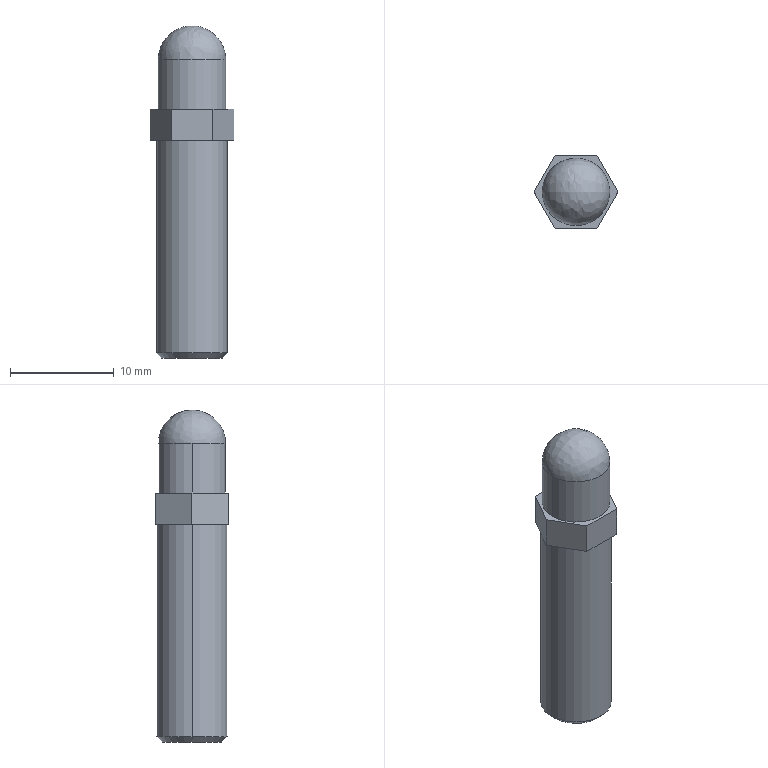Part | STEP file | Product upper | 1 solid | 16 faces | box 8.083 x 7 x 31.87 mm | volume 1117 mm3 | plane 9 | cylinder 4 | cone 2 | spline 1 | commonest cylinder face diameters 6.5 x2 6.8 x2
STEP:
#1=CARTESIAN_POINT('',(0.,0.,0.));
#2=DIRECTION('',(0.,0.,1.));
#3=DIRECTION('',(1.,0.,0.));
#4=AXIS2_PLACEMENT_3D('',#1,#2,#3);
#5=CARTESIAN_POINT('',(3.4,0.,-20.5));
#6=VERTEX_POINT('',#5);
#7=CARTESIAN_POINT('',(-3.4,0.,-20.5));
#8=VERTEX_POINT('',#7);
#9=CARTESIAN_POINT('',(0.,0.,-20.5));
#10=DIRECTION('',(0.,0.,1.));
#11=DIRECTION('',(1.,0.,0.));
#12=AXIS2_PLACEMENT_3D('',#9,#10,#11);
#13=CIRCLE('',#12,3.4);
#14=CARTESIAN_POINT('',(0.,0.,-21.));
#15=DIRECTION('',(0.,0.,1.));
#16=DIRECTION('',(1.,0.,0.));
#17=AXIS2_PLACEMENT_3D('',#14,#15,#16);
#18=CYLINDRICAL_SURFACE('',#17,3.4);
#19=CARTESIAN_POINT('',(0.,0.5));
#20=DIRECTION('',(1.,0.));
#21=VECTOR('',#20,1.);
#22=LINE('',#19,#21);
#23=(GEOMETRIC_REPRESENTATION_CONTEXT(2)PARAMETRIC_REPRESENTATION_CONTEXT()REPRESENTATION_CONTEXT('',''));
#24=DEFINITIONAL_REPRESENTATION('',(#22),#23);
#25=PCURVE('',#18,#24);
#26=CARTESIAN_POINT('',(0.,0.,-20.5));
#27=DIRECTION('',(0.,0.,1.));
#28=DIRECTION('',(1.,0.,0.));
#29=AXIS2_PLACEMENT_3D('',#26,#27,#28);
#30=CONICAL_SURFACE('',#29,3.4,0.7854);
#31=CARTESIAN_POINT('',(0.,0.));
#32=DIRECTION('',(1.,0.));
#33=VECTOR('',#32,1.);
#34=LINE('',#31,#33);
#35=(GEOMETRIC_REPRESENTATION_CONTEXT(2)PARAMETRIC_REPRESENTATION_CONTEXT()REPRESENTATION_CONTEXT('',''));
#36=DEFINITIONAL_REPRESENTATION('',(#34),#35);
#37=PCURVE('',#30,#36);
#38=SURFACE_CURVE('',#13,(#25,#37),.PCURVE_S1.);
#39=EDGE_CURVE('',#6,#8,#38,.T.);
#40=ORIENTED_EDGE('',*,*,#39,.T.);
#41=CARTESIAN_POINT('',(-3.4,0.,0.));
#42=VERTEX_POINT('',#41);
#43=CARTESIAN_POINT('',(-3.4,0.,-21.));
#44=DIRECTION('',(0.,0.,1.));
#45=VECTOR('',#44,1.);
#46=LINE('',#43,#45);
#47=CARTESIAN_POINT('',(3.142,0.));
#48=DIRECTION('',(0.,1.));
#49=VECTOR('',#48,1.);
#50=LINE('',#47,#49);
#51=(GEOMETRIC_REPRESENTATION_CONTEXT(2)PARAMETRIC_REPRESENTATION_CONTEXT()REPRESENTATION_CONTEXT('',''));
#52=DEFINITIONAL_REPRESENTATION('',(#50),#51);
#53=PCURVE('',#18,#52);
#54=CARTESIAN_POINT('',(0.,0.,-21.));
#55=DIRECTION('',(0.,0.,1.));
#56=DIRECTION('',(1.,0.,0.));
#57=AXIS2_PLACEMENT_3D('',#54,#55,#56);
#58=CYLINDRICAL_SURFACE('',#57,3.4);
#59=CARTESIAN_POINT('',(3.142,0.));
#60=DIRECTION('',(0.,1.));
#61=VECTOR('',#60,1.);
#62=LINE('',#59,#61);
#63=(GEOMETRIC_REPRESENTATION_CONTEXT(2)PARAMETRIC_REPRESENTATION_CONTEXT()REPRESENTATION_CONTEXT('',''));
#64=DEFINITIONAL_REPRESENTATION('',(#62),#63);
#65=PCURVE('',#58,#64);
#66=SURFACE_CURVE('',#46,(#53,#65),.PCURVE_S1.);
#67=EDGE_CURVE('',#8,#42,#66,.T.);
#68=ORIENTED_EDGE('',*,*,#67,.T.);
#69=CARTESIAN_POINT('',(3.4,0.,0.));
#70=VERTEX_POINT('',#69);
#71=CARTESIAN_POINT('',(0.,0.,0.));
#72=DIRECTION('',(0.,0.,-1.));
#73=DIRECTION('',(1.,0.,0.));
#74=AXIS2_PLACEMENT_3D('',#71,#72,#73);
#75=CIRCLE('',#74,3.4);
#76=CARTESIAN_POINT('',(6.283,21.));
#77=DIRECTION('',(-1.,0.));
#78=VECTOR('',#77,1.);
#79=LINE('',#76,#78);
#80=(GEOMETRIC_REPRESENTATION_CONTEXT(2)PARAMETRIC_REPRESENTATION_CONTEXT()REPRESENTATION_CONTEXT('',''));
#81=DEFINITIONAL_REPRESENTATION('',(#79),#80);
#82=PCURVE('',#18,#81);
#83=CARTESIAN_POINT('',(0.,0.,0.));
#84=DIRECTION('',(0.,0.,1.));
#85=DIRECTION('',(1.,0.,0.));
#86=AXIS2_PLACEMENT_3D('',#83,#84,#85);
#87=PLANE('',#86);
#88=CARTESIAN_POINT('',(3.4,0.));
#89=CARTESIAN_POINT('',(3.4,-5.889));
#90=CARTESIAN_POINT('',(-1.7,-2.944));
#91=CARTESIAN_POINT('',(-6.8,0.));
#92=CARTESIAN_POINT('',(-1.7,2.944));
#93=CARTESIAN_POINT('',(3.4,5.889));
#94=CARTESIAN_POINT('',(3.4,0.));
#95=(BOUNDED_CURVE()B_SPLINE_CURVE(2,(#88,#89,#90,#91,#92,#93,#94),.UNSPECIFIED.,.T.,.F.)B_SPLINE_CURVE_WITH_KNOTS((1,2,2,2,2,1),(-2.094,0.,2.094,4.189,6.283,8.378),.UNSPECIFIED.)CURVE()GEOMETRIC_REPRESENTATION_ITEM()RATIONAL_B_SPLINE_CURVE((1.,0.5,1.,0.5,1.,0.5,1.))REPRESENTATION_ITEM(''));
#96=(GEOMETRIC_REPRESENTATION_CONTEXT(2)PARAMETRIC_REPRESENTATION_CONTEXT()REPRESENTATION_CONTEXT('',''));
#97=DEFINITIONAL_REPRESENTATION('',(#95),#96);
#98=PCURVE('',#87,#97);
#99=SURFACE_CURVE('',#75,(#82,#98),.PCURVE_S1.);
#100=EDGE_CURVE('',#42,#70,#99,.T.);
#101=ORIENTED_EDGE('',*,*,#100,.T.);
#102=CARTESIAN_POINT('',(3.4,0.,-21.));
#103=DIRECTION('',(0.,0.,1.));
#104=VECTOR('',#103,1.);
#105=LINE('',#102,#104);
#106=CARTESIAN_POINT('',(0.,0.));
#107=DIRECTION('',(0.,1.));
#108=VECTOR('',#107,1.);
#109=LINE('',#106,#108);
#110=(GEOMETRIC_REPRESENTATION_CONTEXT(2)PARAMETRIC_REPRESENTATION_CONTEXT()REPRESENTATION_CONTEXT('',''));
#111=DEFINITIONAL_REPRESENTATION('',(#109),#110);
#112=PCURVE('',#18,#111);
#113=CARTESIAN_POINT('',(6.283,0.));
#114=DIRECTION('',(0.,1.));
#115=VECTOR('',#114,1.);
#116=LINE('',#113,#115);
#117=(GEOMETRIC_REPRESENTATION_CONTEXT(2)PARAMETRIC_REPRESENTATION_CONTEXT()REPRESENTATION_CONTEXT('',''));
#118=DEFINITIONAL_REPRESENTATION('',(#116),#117);
#119=PCURVE('',#58,#118);
#120=SURFACE_CURVE('',#105,(#112,#119),.PCURVE_S1.);
#121=EDGE_CURVE('',#6,#70,#120,.T.);
#122=ORIENTED_EDGE('',*,*,#121,.F.);
#123=EDGE_LOOP('',(#40,#68,#101,#122));
#124=FACE_BOUND('',#123,.T.);
#125=ADVANCED_FACE('',(#124),#18,.T.);
#126=CARTESIAN_POINT('',(2.9,0.,-21.));
#127=VERTEX_POINT('',#126);
#128=CARTESIAN_POINT('',(-2.9,0.,-21.));
#129=VERTEX_POINT('',#128);
#130=CARTESIAN_POINT('',(0.,0.,-21.));
#131=DIRECTION('',(0.,0.,1.));
#132=DIRECTION('',(1.,0.,0.));
#133=AXIS2_PLACEMENT_3D('',#130,#131,#132);
#134=CIRCLE('',#133,2.9);
#135=CARTESIAN_POINT('',(0.,-0.5));
#136=DIRECTION('',(1.,0.));
#137=VECTOR('',#136,1.);
#138=LINE('',#135,#137);
#139=(GEOMETRIC_REPRESENTATION_CONTEXT(2)PARAMETRIC_REPRESENTATION_CONTEXT()REPRESENTATION_CONTEXT('',''));
#140=DEFINITIONAL_REPRESENTATION('',(#138),#139);
#141=PCURVE('',#30,#140);
#142=CARTESIAN_POINT('',(0.,0.,-21.));
#143=DIRECTION('',(0.,0.,-1.));
#144=DIRECTION('',(-1.,0.,0.));
#145=AXIS2_PLACEMENT_3D('',#142,#143,#144);
#146=PLANE('',#145);
#147=CARTESIAN_POINT('',(-2.9,0.));
#148=CARTESIAN_POINT('',(-2.9,5.023));
#149=CARTESIAN_POINT('',(1.45,2.511));
#150=CARTESIAN_POINT('',(5.8,0.));
#151=CARTESIAN_POINT('',(1.45,-2.511));
#152=CARTESIAN_POINT('',(-2.9,-5.023));
#153=CARTESIAN_POINT('',(-2.9,0.));
#154=(BOUNDED_CURVE()B_SPLINE_CURVE(2,(#147,#148,#149,#150,#151,#152,#153),.UNSPECIFIED.,.T.,.F.)B_SPLINE_CURVE_WITH_KNOTS((1,2,2,2,2,1),(-2.094,0.,2.094,4.189,6.283,8.378),.UNSPECIFIED.)CURVE()GEOMETRIC_REPRESENTATION_ITEM()RATIONAL_B_SPLINE_CURVE((1.,0.5,1.,0.5,1.,0.5,1.))REPRESENTATION_ITEM(''));
#155=(GEOMETRIC_REPRESENTATION_CONTEXT(2)PARAMETRIC_REPRESENTATION_CONTEXT()REPRESENTATION_CONTEXT('',''));
#156=DEFINITIONAL_REPRESENTATION('',(#154),#155);
#157=PCURVE('',#146,#156);
#158=SURFACE_CURVE('',#134,(#141,#157),.PCURVE_S1.);
#159=EDGE_CURVE('',#127,#129,#158,.T.);
#160=ORIENTED_EDGE('',*,*,#159,.T.);
#161=CARTESIAN_POINT('',(-3.4,0.,-20.5));
#162=DIRECTION('',(-0.7071,0.,0.7071));
#163=VECTOR('',#162,1.);
#164=LINE('',#161,#163);
#165=CARTESIAN_POINT('',(3.142,0.));
#166=DIRECTION('',(0.,1.));
#167=VECTOR('',#166,1.);
#168=LINE('',#165,#167);
#169=(GEOMETRIC_REPRESENTATION_CONTEXT(2)PARAMETRIC_REPRESENTATION_CONTEXT()REPRESENTATION_CONTEXT('',''));
#170=DEFINITIONAL_REPRESENTATION('',(#168),#169);
#171=PCURVE('',#30,#170);
#172=CARTESIAN_POINT('',(0.,0.,-20.5));
#173=DIRECTION('',(0.,0.,1.));
#174=DIRECTION('',(1.,0.,0.));
#175=AXIS2_PLACEMENT_3D('',#172,#173,#174);
#176=CONICAL_SURFACE('',#175,3.4,0.7854);
#177=CARTESIAN_POINT('',(3.142,0.));
#178=DIRECTION('',(0.,1.));
#179=VECTOR('',#178,1.);
#180=LINE('',#177,#179);
#181=(GEOMETRIC_REPRESENTATION_CONTEXT(2)PARAMETRIC_REPRESENTATION_CONTEXT()REPRESENTATION_CONTEXT('',''));
#182=DEFINITIONAL_REPRESENTATION('',(#180),#181);
#183=PCURVE('',#176,#182);
#184=SURFACE_CURVE('',#164,(#171,#183),.PCURVE_S1.);
#185=EDGE_CURVE('',#129,#8,#184,.T.);
#186=ORIENTED_EDGE('',*,*,#185,.T.);
#187=ORIENTED_EDGE('',*,*,#39,.F.);
#188=CARTESIAN_POINT('',(3.4,0.,-20.5));
#189=DIRECTION('',(0.7071,0.,0.7071));
#190=VECTOR('',#189,1.);
#191=LINE('',#188,#190);
#192=CARTESIAN_POINT('',(0.,0.));
#193=DIRECTION('',(0.,1.));
#194=VECTOR('',#193,1.);
#195=LINE('',#192,#194);
#196=(GEOMETRIC_REPRESENTATION_CONTEXT(2)PARAMETRIC_REPRESENTATION_CONTEXT()REPRESENTATION_CONTEXT('',''));
#197=DEFINITIONAL_REPRESENTATION('',(#195),#196);
#198=PCURVE('',#30,#197);
#199=CARTESIAN_POINT('',(6.283,0.));
#200=DIRECTION('',(0.,1.));
#201=VECTOR('',#200,1.);
#202=LINE('',#199,#201);
#203=(GEOMETRIC_REPRESENTATION_CONTEXT(2)PARAMETRIC_REPRESENTATION_CONTEXT()REPRESENTATION_CONTEXT('',''));
#204=DEFINITIONAL_REPRESENTATION('',(#202),#203);
#205=PCURVE('',#176,#204);
#206=SURFACE_CURVE('',#191,(#198,#205),.PCURVE_S1.);
#207=EDGE_CURVE('',#127,#6,#206,.T.);
#208=ORIENTED_EDGE('',*,*,#207,.F.);
#209=EDGE_LOOP('',(#160,#186,#187,#208));
#210=FACE_BOUND('',#209,.T.);
#211=ADVANCED_FACE('',(#210),#30,.T.);
#212=CARTESIAN_POINT('',(-3.25,0.,7.75));
#213=VERTEX_POINT('',#212);
#214=CARTESIAN_POINT('',(3.25,0.,7.75));
#215=VERTEX_POINT('',#214);
#216=CARTESIAN_POINT('',(0.,0.,7.75));
#217=DIRECTION('',(0.,0.,-1.));
#218=DIRECTION('',(-1.,0.,0.));
#219=AXIS2_PLACEMENT_3D('',#216,#217,#218);
#220=CIRCLE('',#219,3.25);
#221=CARTESIAN_POINT('',(0.,0.,11.));
#222=DIRECTION('',(0.,0.,-1.));
#223=DIRECTION('',(-1.,0.,0.));
#224=AXIS2_PLACEMENT_3D('',#221,#222,#223);
#225=CYLINDRICAL_SURFACE('',#224,3.25);
#226=CARTESIAN_POINT('',(0.,3.25));
#227=DIRECTION('',(1.,0.));
#228=VECTOR('',#227,1.);
#229=LINE('',#226,#228);
#230=(GEOMETRIC_REPRESENTATION_CONTEXT(2)PARAMETRIC_REPRESENTATION_CONTEXT()REPRESENTATION_CONTEXT('',''));
#231=DEFINITIONAL_REPRESENTATION('',(#229),#230);
#232=PCURVE('',#225,#231);
#233=CARTESIAN_POINT('',(3.25,0.,7.75));
#234=CARTESIAN_POINT('',(3.25,0.,7.75));
#235=CARTESIAN_POINT('',(3.25,0.,7.75));
#236=CARTESIAN_POINT('',(3.25,0.,7.75));
#237=CARTESIAN_POINT('',(3.25,6.5,7.75));
#238=CARTESIAN_POINT('',(3.25,6.5,20.75));
#239=CARTESIAN_POINT('',(3.25,-6.5,20.75));
#240=CARTESIAN_POINT('',(3.25,-6.5,7.75));
#241=CARTESIAN_POINT('',(-3.25,6.5,7.75));
#242=CARTESIAN_POINT('',(-3.25,6.5,20.75));
#243=CARTESIAN_POINT('',(-3.25,-6.5,20.75));
#244=CARTESIAN_POINT('',(-3.25,-6.5,7.75));
#245=CARTESIAN_POINT('',(-3.25,0.,7.75));
#246=CARTESIAN_POINT('',(-3.25,0.,7.75));
#247=CARTESIAN_POINT('',(-3.25,0.,7.75));
#248=CARTESIAN_POINT('',(-3.25,0.,7.75));
#249=(BOUNDED_SURFACE()B_SPLINE_SURFACE(3,3,((#233,#234,#235,#236),(#237,#238,#239,#240),(#241,#242,#243,#244),(#245,#246,#247,#248)),.UNSPECIFIED.,.F.,.F.,.F.)B_SPLINE_SURFACE_WITH_KNOTS((4,4),(4,4),(0.,1.),(0.,1.),.PIECEWISE_BEZIER_KNOTS.)GEOMETRIC_REPRESENTATION_ITEM()RATIONAL_B_SPLINE_SURFACE(((1.,0.3333,0.3333,1.),(0.3333,0.1111,0.1111,0.3333),(0.3333,0.1111,0.1111,0.3333),(1.,0.3333,0.3333,1.)))REPRESENTATION_ITEM('')SURFACE());
#250=CARTESIAN_POINT('',(1.,0.));
#251=CARTESIAN_POINT('',(0.9763,0.));
#252=CARTESIAN_POINT('',(0.9319,0.));
#253=CARTESIAN_POINT('',(0.8733,0.));
#254=CARTESIAN_POINT('',(0.8206,0.));
#255=CARTESIAN_POINT('',(0.7724,0.));
#256=CARTESIAN_POINT('',(0.7279,0.));
#257=CARTESIAN_POINT('',(0.6861,0.));
#258=CARTESIAN_POINT('',(0.6465,0.));
#259=CARTESIAN_POINT('',(0.6086,0.));
#260=CARTESIAN_POINT('',(0.5718,0.));
#261=CARTESIAN_POINT('',(0.5357,0.));
#262=CARTESIAN_POINT('',(0.5,0.));
#263=CARTESIAN_POINT('',(0.4643,0.));
#264=CARTESIAN_POINT('',(0.4282,0.));
#265=CARTESIAN_POINT('',(0.3914,0.));
#266=CARTESIAN_POINT('',(0.3535,0.));
#267=CARTESIAN_POINT('',(0.3139,0.));
#268=CARTESIAN_POINT('',(0.2721,0.));
#269=CARTESIAN_POINT('',(0.2276,0.));
#270=CARTESIAN_POINT('',(0.1794,0.));
#271=CARTESIAN_POINT('',(0.1267,0.));
#272=CARTESIAN_POINT('',(0.06805,0.));
#273=CARTESIAN_POINT('',(0.02375,0.));
#274=CARTESIAN_POINT('',(0.,0.));
#275=B_SPLINE_CURVE_WITH_KNOTS('',3,(#250,#251,#252,#253,#254,#255,#256,#257,#258,#259,#260,#261,#262,#263,#264,#265,#266,#267,#268,#269,#270,#271,#272,#273,#274),.UNSPECIFIED.,.F.,.F.,(4,1,1,1,1,1,1,1,1,1,1,1,1,1,1,1,1,1,1,1,1,1,4),(0.,0.1428,0.2856,0.4284,0.5712,0.714,0.8568,0.9996,1.142,1.285,1.428,1.571,1.714,1.856,1.999,2.142,2.285,2.428,2.57,2.713,2.856,2.999,3.142),.QUASI_UNIFORM_KNOTS.);
#276=(GEOMETRIC_REPRESENTATION_CONTEXT(2)PARAMETRIC_REPRESENTATION_CONTEXT()REPRESENTATION_CONTEXT('',''));
#277=DEFINITIONAL_REPRESENTATION('',(#275),#276);
#278=PCURVE('',#249,#277);
#279=SURFACE_CURVE('',#220,(#232,#278),.PCURVE_S1.);
#280=EDGE_CURVE('',#213,#215,#279,.T.);
#281=ORIENTED_EDGE('',*,*,#280,.T.);
#282=CARTESIAN_POINT('',(3.25,0.,3.));
#283=VERTEX_POINT('',#282);
#284=CARTESIAN_POINT('',(3.25,0.,11.));
#285=DIRECTION('',(0.,0.,-1.));
#286=VECTOR('',#285,1.);
#287=LINE('',#284,#286);
#288=CARTESIAN_POINT('',(3.142,0.));
#289=DIRECTION('',(0.,1.));
#290=VECTOR('',#289,1.);
#291=LINE('',#288,#290);
#292=(GEOMETRIC_REPRESENTATION_CONTEXT(2)PARAMETRIC_REPRESENTATION_CONTEXT()REPRESENTATION_CONTEXT('',''));
#293=DEFINITIONAL_REPRESENTATION('',(#291),#292);
#294=PCURVE('',#225,#293);
#295=CARTESIAN_POINT('',(0.,0.,11.));
#296=DIRECTION('',(0.,0.,-1.));
#297=DIRECTION('',(-1.,0.,0.));
#298=AXIS2_PLACEMENT_3D('',#295,#296,#297);
#299=CYLINDRICAL_SURFACE('',#298,3.25);
#300=CARTESIAN_POINT('',(3.142,0.));
#301=DIRECTION('',(0.,1.));
#302=VECTOR('',#301,1.);
#303=LINE('',#300,#302);
#304=(GEOMETRIC_REPRESENTATION_CONTEXT(2)PARAMETRIC_REPRESENTATION_CONTEXT()REPRESENTATION_CONTEXT('',''));
#305=DEFINITIONAL_REPRESENTATION('',(#303),#304);
#306=PCURVE('',#299,#305);
#307=SURFACE_CURVE('',#287,(#294,#306),.PCURVE_S1.);
#308=EDGE_CURVE('',#215,#283,#307,.T.);
#309=ORIENTED_EDGE('',*,*,#308,.T.);
#310=CARTESIAN_POINT('',(-3.25,0.,3.));
#311=VERTEX_POINT('',#310);
#312=CARTESIAN_POINT('',(0.,0.,3.));
#313=DIRECTION('',(0.,0.,-1.));
#314=DIRECTION('',(-1.,0.,0.));
#315=AXIS2_PLACEMENT_3D('',#312,#313,#314);
#316=CIRCLE('',#315,3.25);
#317=CARTESIAN_POINT('',(0.,8.));
#318=DIRECTION('',(1.,0.));
#319=VECTOR('',#318,1.);
#320=LINE('',#317,#319);
#321=(GEOMETRIC_REPRESENTATION_CONTEXT(2)PARAMETRIC_REPRESENTATION_CONTEXT()REPRESENTATION_CONTEXT('',''));
#322=DEFINITIONAL_REPRESENTATION('',(#320),#321);
#323=PCURVE('',#225,#322);
#324=CARTESIAN_POINT('',(0.,0.,3.));
#325=DIRECTION('',(0.,0.,1.));
#326=DIRECTION('',(1.,0.,0.));
#327=AXIS2_PLACEMENT_3D('',#324,#325,#326);
#328=PLANE('',#327);
#329=CARTESIAN_POINT('',(-3.25,0.));
#330=CARTESIAN_POINT('',(-3.25,5.629));
#331=CARTESIAN_POINT('',(1.625,2.815));
#332=CARTESIAN_POINT('',(6.5,0.));
#333=CARTESIAN_POINT('',(1.625,-2.815));
#334=CARTESIAN_POINT('',(-3.25,-5.629));
#335=CARTESIAN_POINT('',(-3.25,0.));
#336=(BOUNDED_CURVE()B_SPLINE_CURVE(2,(#329,#330,#331,#332,#333,#334,#335),.UNSPECIFIED.,.T.,.F.)B_SPLINE_CURVE_WITH_KNOTS((1,2,2,2,2,1),(-2.094,0.,2.094,4.189,6.283,8.378),.UNSPECIFIED.)CURVE()GEOMETRIC_REPRESENTATION_ITEM()RATIONAL_B_SPLINE_CURVE((1.,0.5,1.,0.5,1.,0.5,1.))REPRESENTATION_ITEM(''));
#337=(GEOMETRIC_REPRESENTATION_CONTEXT(2)PARAMETRIC_REPRESENTATION_CONTEXT()REPRESENTATION_CONTEXT('',''));
#338=DEFINITIONAL_REPRESENTATION('',(#336),#337);
#339=PCURVE('',#328,#338);
#340=SURFACE_CURVE('',#316,(#323,#339),.PCURVE_S1.);
#341=EDGE_CURVE('',#311,#283,#340,.T.);
#342=ORIENTED_EDGE('',*,*,#341,.F.);
#343=CARTESIAN_POINT('',(-3.25,0.,11.));
#344=DIRECTION('',(0.,0.,-1.));
#345=VECTOR('',#344,1.);
#346=LINE('',#343,#345);
#347=CARTESIAN_POINT('',(0.,0.));
#348=DIRECTION('',(0.,1.));
#349=VECTOR('',#348,1.);
#350=LINE('',#347,#349);
#351=(GEOMETRIC_REPRESENTATION_CONTEXT(2)PARAMETRIC_REPRESENTATION_CONTEXT()REPRESENTATION_CONTEXT('',''));
#352=DEFINITIONAL_REPRESENTATION('',(#350),#351);
#353=PCURVE('',#225,#352);
#354=CARTESIAN_POINT('',(6.283,0.));
#355=DIRECTION('',(0.,1.));
#356=VECTOR('',#355,1.);
#357=LINE('',#354,#356);
#358=(GEOMETRIC_REPRESENTATION_CONTEXT(2)PARAMETRIC_REPRESENTATION_CONTEXT()REPRESENTATION_CONTEXT('',''));
#359=DEFINITIONAL_REPRESENTATION('',(#357),#358);
#360=PCURVE('',#299,#359);
#361=SURFACE_CURVE('',#346,(#353,#360),.PCURVE_S1.);
#362=EDGE_CURVE('',#213,#311,#361,.T.);
#363=ORIENTED_EDGE('',*,*,#362,.F.);
#364=EDGE_LOOP('',(#281,#309,#342,#363));
#365=FACE_BOUND('',#364,.T.);
#366=ADVANCED_FACE('',(#365),#225,.T.);
#367=ORIENTED_EDGE('',*,*,#67,.F.);
#368=CARTESIAN_POINT('',(0.,0.,-20.5));
#369=DIRECTION('',(0.,0.,1.));
#370=DIRECTION('',(1.,0.,0.));
#371=AXIS2_PLACEMENT_3D('',#368,#369,#370);
#372=CIRCLE('',#371,3.4);
#373=CARTESIAN_POINT('',(0.,0.5));
#374=DIRECTION('',(1.,0.));
#375=VECTOR('',#374,1.);
#376=LINE('',#373,#375);
#377=(GEOMETRIC_REPRESENTATION_CONTEXT(2)PARAMETRIC_REPRESENTATION_CONTEXT()REPRESENTATION_CONTEXT('',''));
#378=DEFINITIONAL_REPRESENTATION('',(#376),#377);
#379=PCURVE('',#58,#378);
#380=CARTESIAN_POINT('',(0.,0.));
#381=DIRECTION('',(1.,0.));
#382=VECTOR('',#381,1.);
#383=LINE('',#380,#382);
#384=(GEOMETRIC_REPRESENTATION_CONTEXT(2)PARAMETRIC_REPRESENTATION_CONTEXT()REPRESENTATION_CONTEXT('',''));
#385=DEFINITIONAL_REPRESENTATION('',(#383),#384);
#386=PCURVE('',#176,#385);
#387=SURFACE_CURVE('',#372,(#379,#386),.PCURVE_S1.);
#388=EDGE_CURVE('',#8,#6,#387,.T.);
#389=ORIENTED_EDGE('',*,*,#388,.T.);
#390=ORIENTED_EDGE('',*,*,#121,.T.);
#391=CARTESIAN_POINT('',(0.,0.,0.));
#392=DIRECTION('',(0.,0.,-1.));
#393=DIRECTION('',(1.,0.,0.));
#394=AXIS2_PLACEMENT_3D('',#391,#392,#393);
#395=CIRCLE('',#394,3.4);
#396=CARTESIAN_POINT('',(6.283,21.));
#397=DIRECTION('',(-1.,0.));
#398=VECTOR('',#397,1.);
#399=LINE('',#396,#398);
#400=(GEOMETRIC_REPRESENTATION_CONTEXT(2)PARAMETRIC_REPRESENTATION_CONTEXT()REPRESENTATION_CONTEXT('',''));
#401=DEFINITIONAL_REPRESENTATION('',(#399),#400);
#402=PCURVE('',#58,#401);
#403=CARTESIAN_POINT('',(3.4,0.));
#404=CARTESIAN_POINT('',(3.4,-5.889));
#405=CARTESIAN_POINT('',(-1.7,-2.944));
#406=CARTESIAN_POINT('',(-6.8,0.));
#407=CARTESIAN_POINT('',(-1.7,2.944));
#408=CARTESIAN_POINT('',(3.4,5.889));
#409=CARTESIAN_POINT('',(3.4,0.));
#410=(BOUNDED_CURVE()B_SPLINE_CURVE(2,(#403,#404,#405,#406,#407,#408,#409),.UNSPECIFIED.,.T.,.F.)B_SPLINE_CURVE_WITH_KNOTS((1,2,2,2,2,1),(-2.094,0.,2.094,4.189,6.283,8.378),.UNSPECIFIED.)CURVE()GEOMETRIC_REPRESENTATION_ITEM()RATIONAL_B_SPLINE_CURVE((1.,0.5,1.,0.5,1.,0.5,1.))REPRESENTATION_ITEM(''));
#411=(GEOMETRIC_REPRESENTATION_CONTEXT(2)PARAMETRIC_REPRESENTATION_CONTEXT()REPRESENTATION_CONTEXT('',''));
#412=DEFINITIONAL_REPRESENTATION('',(#410),#411);
#413=PCURVE('',#87,#412);
#414=SURFACE_CURVE('',#395,(#402,#413),.PCURVE_S1.);
#415=EDGE_CURVE('',#70,#42,#414,.T.);
#416=ORIENTED_EDGE('',*,*,#415,.T.);
#417=EDGE_LOOP('',(#367,#389,#390,#416));
#418=FACE_BOUND('',#417,.T.);
#419=ADVANCED_FACE('',(#418),#58,.T.);
#420=ORIENTED_EDGE('',*,*,#415,.F.);
#421=ORIENTED_EDGE('',*,*,#100,.F.);
#422=EDGE_LOOP('',(#420,#421));
#423=FACE_BOUND('',#422,.T.);
#424=CARTESIAN_POINT('',(-2.021,-3.5,0.));
#425=VERTEX_POINT('',#424);
#426=CARTESIAN_POINT('',(2.021,-3.5,0.));
#427=VERTEX_POINT('',#426);
#428=CARTESIAN_POINT('',(0.,-3.5,0.));
#429=DIRECTION('',(1.,0.,0.));
#430=VECTOR('',#429,1.);
#431=LINE('',#428,#430);
#432=CARTESIAN_POINT('',(0.,-3.5));
#433=DIRECTION('',(1.,0.));
#434=VECTOR('',#433,1.);
#435=LINE('',#432,#434);
#436=(GEOMETRIC_REPRESENTATION_CONTEXT(2)PARAMETRIC_REPRESENTATION_CONTEXT()REPRESENTATION_CONTEXT('',''));
#437=DEFINITIONAL_REPRESENTATION('',(#435),#436);
#438=PCURVE('',#87,#437);
#439=CARTESIAN_POINT('',(-2.021,-3.5,3.));
#440=DIRECTION('',(0.,1.,0.));
#441=DIRECTION('',(-1.,0.,0.));
#442=AXIS2_PLACEMENT_3D('',#439,#440,#441);
#443=PLANE('',#442);
#444=CARTESIAN_POINT('',(-2.021,-3.));
#445=DIRECTION('',(-1.,0.));
#446=VECTOR('',#445,1.);
#447=LINE('',#444,#446);
#448=(GEOMETRIC_REPRESENTATION_CONTEXT(2)PARAMETRIC_REPRESENTATION_CONTEXT()REPRESENTATION_CONTEXT('',''));
#449=DEFINITIONAL_REPRESENTATION('',(#447),#448);
#450=PCURVE('',#443,#449);
#451=SURFACE_CURVE('',#431,(#438,#450),.PCURVE_S1.);
#452=EDGE_CURVE('',#425,#427,#451,.T.);
#453=ORIENTED_EDGE('',*,*,#452,.F.);
#454=CARTESIAN_POINT('',(-4.041,0.,0.));
#455=VERTEX_POINT('',#454);
#456=CARTESIAN_POINT('',(-4.041,0.,0.));
#457=DIRECTION('',(0.5,-0.866,0.));
#458=VECTOR('',#457,1.);
#459=LINE('',#456,#458);
#460=CARTESIAN_POINT('',(-4.041,0.));
#461=DIRECTION('',(0.5,-0.866));
#462=VECTOR('',#461,1.);
#463=LINE('',#460,#462);
#464=(GEOMETRIC_REPRESENTATION_CONTEXT(2)PARAMETRIC_REPRESENTATION_CONTEXT()REPRESENTATION_CONTEXT('',''));
#465=DEFINITIONAL_REPRESENTATION('',(#463),#464);
#466=PCURVE('',#87,#465);
#467=CARTESIAN_POINT('',(-4.041,0.,3.));
#468=DIRECTION('',(0.866,0.5,0.));
#469=DIRECTION('',(-0.5,0.866,0.));
#470=AXIS2_PLACEMENT_3D('',#467,#468,#469);
#471=PLANE('',#470);
#472=CARTESIAN_POINT('',(0.,-3.));
#473=DIRECTION('',(-1.,0.));
#474=VECTOR('',#473,1.);
#475=LINE('',#472,#474);
#476=(GEOMETRIC_REPRESENTATION_CONTEXT(2)PARAMETRIC_REPRESENTATION_CONTEXT()REPRESENTATION_CONTEXT('',''));
#477=DEFINITIONAL_REPRESENTATION('',(#475),#476);
#478=PCURVE('',#471,#477);
#479=SURFACE_CURVE('',#459,(#466,#478),.PCURVE_S1.);
#480=EDGE_CURVE('',#455,#425,#479,.T.);
#481=ORIENTED_EDGE('',*,*,#480,.F.);
#482=CARTESIAN_POINT('',(-2.021,3.5,0.));
#483=VERTEX_POINT('',#482);
#484=CARTESIAN_POINT('',(-2.021,3.5,0.));
#485=DIRECTION('',(-0.5,-0.866,0.));
#486=VECTOR('',#485,1.);
#487=LINE('',#484,#486);
#488=CARTESIAN_POINT('',(-2.021,3.5));
#489=DIRECTION('',(-0.5,-0.866));
#490=VECTOR('',#489,1.);
#491=LINE('',#488,#490);
#492=(GEOMETRIC_REPRESENTATION_CONTEXT(2)PARAMETRIC_REPRESENTATION_CONTEXT()REPRESENTATION_CONTEXT('',''));
#493=DEFINITIONAL_REPRESENTATION('',(#491),#492);
#494=PCURVE('',#87,#493);
#495=CARTESIAN_POINT('',(-2.021,3.5,3.));
#496=DIRECTION('',(0.866,-0.5,0.));
#497=DIRECTION('',(0.5,0.866,0.));
#498=AXIS2_PLACEMENT_3D('',#495,#496,#497);
#499=PLANE('',#498);
#500=CARTESIAN_POINT('',(0.,-3.));
#501=DIRECTION('',(-1.,0.));
#502=VECTOR('',#501,1.);
#503=LINE('',#500,#502);
#504=(GEOMETRIC_REPRESENTATION_CONTEXT(2)PARAMETRIC_REPRESENTATION_CONTEXT()REPRESENTATION_CONTEXT('',''));
#505=DEFINITIONAL_REPRESENTATION('',(#503),#504);
#506=PCURVE('',#499,#505);
#507=SURFACE_CURVE('',#487,(#494,#506),.PCURVE_S1.);
#508=EDGE_CURVE('',#483,#455,#507,.T.);
#509=ORIENTED_EDGE('',*,*,#508,.F.);
#510=CARTESIAN_POINT('',(2.021,3.5,0.));
#511=VERTEX_POINT('',#510);
#512=CARTESIAN_POINT('',(0.,3.5,0.));
#513=DIRECTION('',(-1.,0.,0.));
#514=VECTOR('',#513,1.);
#515=LINE('',#512,#514);
#516=CARTESIAN_POINT('',(0.,3.5));
#517=DIRECTION('',(-1.,0.));
#518=VECTOR('',#517,1.);
#519=LINE('',#516,#518);
#520=(GEOMETRIC_REPRESENTATION_CONTEXT(2)PARAMETRIC_REPRESENTATION_CONTEXT()REPRESENTATION_CONTEXT('',''));
#521=DEFINITIONAL_REPRESENTATION('',(#519),#520);
#522=PCURVE('',#87,#521);
#523=CARTESIAN_POINT('',(2.021,3.5,3.));
#524=DIRECTION('',(0.,-1.,0.));
#525=DIRECTION('',(0.,0.,-1.));
#526=AXIS2_PLACEMENT_3D('',#523,#524,#525);
#527=PLANE('',#526);
#528=CARTESIAN_POINT('',(3.,-2.021));
#529=DIRECTION('',(0.,-1.));
#530=VECTOR('',#529,1.);
#531=LINE('',#528,#530);
#532=(GEOMETRIC_REPRESENTATION_CONTEXT(2)PARAMETRIC_REPRESENTATION_CONTEXT()REPRESENTATION_CONTEXT('',''));
#533=DEFINITIONAL_REPRESENTATION('',(#531),#532);
#534=PCURVE('',#527,#533);
#535=SURFACE_CURVE('',#515,(#522,#534),.PCURVE_S1.);
#536=EDGE_CURVE('',#511,#483,#535,.T.);
#537=ORIENTED_EDGE('',*,*,#536,.F.);
#538=CARTESIAN_POINT('',(4.041,0.,0.));
#539=VERTEX_POINT('',#538);
#540=CARTESIAN_POINT('',(4.041,0.,0.));
#541=DIRECTION('',(-0.5,0.866,0.));
#542=VECTOR('',#541,1.);
#543=LINE('',#540,#542);
#544=CARTESIAN_POINT('',(4.041,0.));
#545=DIRECTION('',(-0.5,0.866));
#546=VECTOR('',#545,1.);
#547=LINE('',#544,#546);
#548=(GEOMETRIC_REPRESENTATION_CONTEXT(2)PARAMETRIC_REPRESENTATION_CONTEXT()REPRESENTATION_CONTEXT('',''));
#549=DEFINITIONAL_REPRESENTATION('',(#547),#548);
#550=PCURVE('',#87,#549);
#551=CARTESIAN_POINT('',(4.041,0.,3.));
#552=DIRECTION('',(-0.866,-0.5,0.));
#553=DIRECTION('',(0.5,-0.866,0.));
#554=AXIS2_PLACEMENT_3D('',#551,#552,#553);
#555=PLANE('',#554);
#556=CARTESIAN_POINT('',(0.,-3.));
#557=DIRECTION('',(-1.,0.));
#558=VECTOR('',#557,1.);
#559=LINE('',#556,#558);
#560=(GEOMETRIC_REPRESENTATION_CONTEXT(2)PARAMETRIC_REPRESENTATION_CONTEXT()REPRESENTATION_CONTEXT('',''));
#561=DEFINITIONAL_REPRESENTATION('',(#559),#560);
#562=PCURVE('',#555,#561);
#563=SURFACE_CURVE('',#543,(#550,#562),.PCURVE_S1.);
#564=EDGE_CURVE('',#539,#511,#563,.T.);
#565=ORIENTED_EDGE('',*,*,#564,.F.);
#566=CARTESIAN_POINT('',(2.021,-3.5,0.));
#567=DIRECTION('',(0.5,0.866,0.));
#568=VECTOR('',#567,1.);
#569=LINE('',#566,#568);
#570=CARTESIAN_POINT('',(2.021,-3.5));
#571=DIRECTION('',(0.5,0.866));
#572=VECTOR('',#571,1.);
#573=LINE('',#570,#572);
#574=(GEOMETRIC_REPRESENTATION_CONTEXT(2)PARAMETRIC_REPRESENTATION_CONTEXT()REPRESENTATION_CONTEXT('',''));
#575=DEFINITIONAL_REPRESENTATION('',(#573),#574);
#576=PCURVE('',#87,#575);
#577=CARTESIAN_POINT('',(2.021,-3.5,3.));
#578=DIRECTION('',(-0.866,0.5,0.));
#579=DIRECTION('',(-0.5,-0.866,0.));
#580=AXIS2_PLACEMENT_3D('',#577,#578,#579);
#581=PLANE('',#580);
#582=CARTESIAN_POINT('',(0.,-3.));
#583=DIRECTION('',(-1.,0.));
#584=VECTOR('',#583,1.);
#585=LINE('',#582,#584);
#586=(GEOMETRIC_REPRESENTATION_CONTEXT(2)PARAMETRIC_REPRESENTATION_CONTEXT()REPRESENTATION_CONTEXT('',''));
#587=DEFINITIONAL_REPRESENTATION('',(#585),#586);
#588=PCURVE('',#581,#587);
#589=SURFACE_CURVE('',#569,(#576,#588),.PCURVE_S1.);
#590=EDGE_CURVE('',#427,#539,#589,.T.);
#591=ORIENTED_EDGE('',*,*,#590,.F.);
#592=EDGE_LOOP('',(#453,#481,#509,#537,#565,#591));
#593=FACE_BOUND('',#592,.T.);
#594=ADVANCED_FACE('',(#423,#593),#87,.F.);
#595=ORIENTED_EDGE('',*,*,#185,.F.);
#596=CARTESIAN_POINT('',(0.,0.,-21.));
#597=DIRECTION('',(0.,0.,1.));
#598=DIRECTION('',(1.,0.,0.));
#599=AXIS2_PLACEMENT_3D('',#596,#597,#598);
#600=CIRCLE('',#599,2.9);
#601=CARTESIAN_POINT('',(0.,-0.5));
#602=DIRECTION('',(1.,0.));
#603=VECTOR('',#602,1.);
#604=LINE('',#601,#603);
#605=(GEOMETRIC_REPRESENTATION_CONTEXT(2)PARAMETRIC_REPRESENTATION_CONTEXT()REPRESENTATION_CONTEXT('',''));
#606=DEFINITIONAL_REPRESENTATION('',(#604),#605);
#607=PCURVE('',#176,#606);
#608=CARTESIAN_POINT('',(-2.9,0.));
#609=CARTESIAN_POINT('',(-2.9,5.023));
#610=CARTESIAN_POINT('',(1.45,2.511));
#611=CARTESIAN_POINT('',(5.8,0.));
#612=CARTESIAN_POINT('',(1.45,-2.511));
#613=CARTESIAN_POINT('',(-2.9,-5.023));
#614=CARTESIAN_POINT('',(-2.9,0.));
#615=(BOUNDED_CURVE()B_SPLINE_CURVE(2,(#608,#609,#610,#611,#612,#613,#614),.UNSPECIFIED.,.T.,.F.)B_SPLINE_CURVE_WITH_KNOTS((1,2,2,2,2,1),(-2.094,0.,2.094,4.189,6.283,8.378),.UNSPECIFIED.)CURVE()GEOMETRIC_REPRESENTATION_ITEM()RATIONAL_B_SPLINE_CURVE((1.,0.5,1.,0.5,1.,0.5,1.))REPRESENTATION_ITEM(''));
#616=(GEOMETRIC_REPRESENTATION_CONTEXT(2)PARAMETRIC_REPRESENTATION_CONTEXT()REPRESENTATION_CONTEXT('',''));
#617=DEFINITIONAL_REPRESENTATION('',(#615),#616);
#618=PCURVE('',#146,#617);
#619=SURFACE_CURVE('',#600,(#607,#618),.PCURVE_S1.);
#620=EDGE_CURVE('',#129,#127,#619,.T.);
#621=ORIENTED_EDGE('',*,*,#620,.T.);
#622=ORIENTED_EDGE('',*,*,#207,.T.);
#623=ORIENTED_EDGE('',*,*,#388,.F.);
#624=EDGE_LOOP('',(#595,#621,#622,#623));
#625=FACE_BOUND('',#624,.T.);
#626=ADVANCED_FACE('',(#625),#176,.T.);
#627=CARTESIAN_POINT('',(4.041,0.,3.));
#628=VERTEX_POINT('',#627);
#629=CARTESIAN_POINT('',(4.041,0.,3.));
#630=DIRECTION('',(0.,0.,-1.));
#631=VECTOR('',#630,1.);
#632=LINE('',#629,#631);
#633=CARTESIAN_POINT('',(-4.041,0.));
#634=DIRECTION('',(0.,-1.));
#635=VECTOR('',#634,1.);
#636=LINE('',#633,#635);
#637=(GEOMETRIC_REPRESENTATION_CONTEXT(2)PARAMETRIC_REPRESENTATION_CONTEXT()REPRESENTATION_CONTEXT('',''));
#638=DEFINITIONAL_REPRESENTATION('',(#636),#637);
#639=PCURVE('',#581,#638);
#640=CARTESIAN_POINT('',(0.,0.));
#641=DIRECTION('',(0.,-1.));
#642=VECTOR('',#641,1.);
#643=LINE('',#640,#642);
#644=(GEOMETRIC_REPRESENTATION_CONTEXT(2)PARAMETRIC_REPRESENTATION_CONTEXT()REPRESENTATION_CONTEXT('',''));
#645=DEFINITIONAL_REPRESENTATION('',(#643),#644);
#646=PCURVE('',#555,#645);
#647=SURFACE_CURVE('',#632,(#639,#646),.PCURVE_S1.);
#648=EDGE_CURVE('',#628,#539,#647,.T.);
#649=ORIENTED_EDGE('',*,*,#648,.F.);
#650=CARTESIAN_POINT('',(2.021,-3.5,3.));
#651=VERTEX_POINT('',#650);
#652=CARTESIAN_POINT('',(2.021,-3.5,3.));
#653=DIRECTION('',(0.5,0.866,0.));
#654=VECTOR('',#653,1.);
#655=LINE('',#652,#654);
#656=CARTESIAN_POINT('',(0.,0.));
#657=DIRECTION('',(-1.,0.));
#658=VECTOR('',#657,1.);
#659=LINE('',#656,#658);
#660=(GEOMETRIC_REPRESENTATION_CONTEXT(2)PARAMETRIC_REPRESENTATION_CONTEXT()REPRESENTATION_CONTEXT('',''));
#661=DEFINITIONAL_REPRESENTATION('',(#659),#660);
#662=PCURVE('',#581,#661);
#663=CARTESIAN_POINT('',(2.021,-3.5));
#664=DIRECTION('',(0.5,0.866));
#665=VECTOR('',#664,1.);
#666=LINE('',#663,#665);
#667=(GEOMETRIC_REPRESENTATION_CONTEXT(2)PARAMETRIC_REPRESENTATION_CONTEXT()REPRESENTATION_CONTEXT('',''));
#668=DEFINITIONAL_REPRESENTATION('',(#666),#667);
#669=PCURVE('',#328,#668);
#670=SURFACE_CURVE('',#655,(#662,#669),.PCURVE_S1.);
#671=EDGE_CURVE('',#651,#628,#670,.T.);
#672=ORIENTED_EDGE('',*,*,#671,.F.);
#673=CARTESIAN_POINT('',(2.021,-3.5,3.));
#674=DIRECTION('',(0.,0.,1.));
#675=VECTOR('',#674,1.);
#676=LINE('',#673,#675);
#677=CARTESIAN_POINT('',(0.,0.));
#678=DIRECTION('',(0.,1.));
#679=VECTOR('',#678,1.);
#680=LINE('',#677,#679);
#681=(GEOMETRIC_REPRESENTATION_CONTEXT(2)PARAMETRIC_REPRESENTATION_CONTEXT()REPRESENTATION_CONTEXT('',''));
#682=DEFINITIONAL_REPRESENTATION('',(#680),#681);
#683=PCURVE('',#581,#682);
#684=CARTESIAN_POINT('',(-4.041,0.));
#685=DIRECTION('',(0.,1.));
#686=VECTOR('',#685,1.);
#687=LINE('',#684,#686);
#688=(GEOMETRIC_REPRESENTATION_CONTEXT(2)PARAMETRIC_REPRESENTATION_CONTEXT()REPRESENTATION_CONTEXT('',''));
#689=DEFINITIONAL_REPRESENTATION('',(#687),#688);
#690=PCURVE('',#443,#689);
#691=SURFACE_CURVE('',#676,(#683,#690),.PCURVE_S1.);
#692=EDGE_CURVE('',#427,#651,#691,.T.);
#693=ORIENTED_EDGE('',*,*,#692,.F.);
#694=ORIENTED_EDGE('',*,*,#590,.T.);
#695=EDGE_LOOP('',(#649,#672,#693,#694));
#696=FACE_BOUND('',#695,.T.);
#697=ADVANCED_FACE('',(#696),#581,.F.);
#698=ORIENTED_EDGE('',*,*,#692,.T.);
#699=CARTESIAN_POINT('',(-2.021,-3.5,3.));
#700=VERTEX_POINT('',#699);
#701=CARTESIAN_POINT('',(-2.021,-3.5,3.));
#702=DIRECTION('',(1.,0.,0.));
#703=VECTOR('',#702,1.);
#704=LINE('',#701,#703);
#705=CARTESIAN_POINT('',(0.,0.));
#706=DIRECTION('',(-1.,0.));
#707=VECTOR('',#706,1.);
#708=LINE('',#705,#707);
#709=(GEOMETRIC_REPRESENTATION_CONTEXT(2)PARAMETRIC_REPRESENTATION_CONTEXT()REPRESENTATION_CONTEXT('',''));
#710=DEFINITIONAL_REPRESENTATION('',(#708),#709);
#711=PCURVE('',#443,#710);
#712=CARTESIAN_POINT('',(-2.021,-3.5));
#713=DIRECTION('',(1.,0.));
#714=VECTOR('',#713,1.);
#715=LINE('',#712,#714);
#716=(GEOMETRIC_REPRESENTATION_CONTEXT(2)PARAMETRIC_REPRESENTATION_CONTEXT()REPRESENTATION_CONTEXT('',''));
#717=DEFINITIONAL_REPRESENTATION('',(#715),#716);
#718=PCURVE('',#328,#717);
#719=SURFACE_CURVE('',#704,(#711,#718),.PCURVE_S1.);
#720=EDGE_CURVE('',#700,#651,#719,.T.);
#721=ORIENTED_EDGE('',*,*,#720,.F.);
#722=CARTESIAN_POINT('',(-2.021,-3.5,3.));
#723=DIRECTION('',(0.,0.,1.));
#724=VECTOR('',#723,1.);
#725=LINE('',#722,#724);
#726=CARTESIAN_POINT('',(0.,0.));
#727=DIRECTION('',(0.,1.));
#728=VECTOR('',#727,1.);
#729=LINE('',#726,#728);
#730=(GEOMETRIC_REPRESENTATION_CONTEXT(2)PARAMETRIC_REPRESENTATION_CONTEXT()REPRESENTATION_CONTEXT('',''));
#731=DEFINITIONAL_REPRESENTATION('',(#729),#730);
#732=PCURVE('',#443,#731);
#733=CARTESIAN_POINT('',(-4.041,0.));
#734=DIRECTION('',(0.,1.));
#735=VECTOR('',#734,1.);
#736=LINE('',#733,#735);
#737=(GEOMETRIC_REPRESENTATION_CONTEXT(2)PARAMETRIC_REPRESENTATION_CONTEXT()REPRESENTATION_CONTEXT('',''));
#738=DEFINITIONAL_REPRESENTATION('',(#736),#737);
#739=PCURVE('',#471,#738);
#740=SURFACE_CURVE('',#725,(#732,#739),.PCURVE_S1.);
#741=EDGE_CURVE('',#425,#700,#740,.T.);
#742=ORIENTED_EDGE('',*,*,#741,.F.);
#743=ORIENTED_EDGE('',*,*,#452,.T.);
#744=EDGE_LOOP('',(#698,#721,#742,#743));
#745=FACE_BOUND('',#744,.T.);
#746=ADVANCED_FACE('',(#745),#443,.F.);
#747=ORIENTED_EDGE('',*,*,#741,.T.);
#748=CARTESIAN_POINT('',(-4.041,0.,3.));
#749=VERTEX_POINT('',#748);
#750=CARTESIAN_POINT('',(-4.041,0.,3.));
#751=DIRECTION('',(0.5,-0.866,0.));
#752=VECTOR('',#751,1.);
#753=LINE('',#750,#752);
#754=CARTESIAN_POINT('',(0.,0.));
#755=DIRECTION('',(-1.,0.));
#756=VECTOR('',#755,1.);
#757=LINE('',#754,#756);
#758=(GEOMETRIC_REPRESENTATION_CONTEXT(2)PARAMETRIC_REPRESENTATION_CONTEXT()REPRESENTATION_CONTEXT('',''));
#759=DEFINITIONAL_REPRESENTATION('',(#757),#758);
#760=PCURVE('',#471,#759);
#761=CARTESIAN_POINT('',(-4.041,0.));
#762=DIRECTION('',(0.5,-0.866));
#763=VECTOR('',#762,1.);
#764=LINE('',#761,#763);
#765=(GEOMETRIC_REPRESENTATION_CONTEXT(2)PARAMETRIC_REPRESENTATION_CONTEXT()REPRESENTATION_CONTEXT('',''));
#766=DEFINITIONAL_REPRESENTATION('',(#764),#765);
#767=PCURVE('',#328,#766);
#768=SURFACE_CURVE('',#753,(#760,#767),.PCURVE_S1.);
#769=EDGE_CURVE('',#749,#700,#768,.T.);
#770=ORIENTED_EDGE('',*,*,#769,.F.);
#771=CARTESIAN_POINT('',(-4.041,0.,3.));
#772=DIRECTION('',(0.,0.,1.));
#773=VECTOR('',#772,1.);
#774=LINE('',#771,#773);
#775=CARTESIAN_POINT('',(0.,0.));
#776=DIRECTION('',(0.,1.));
#777=VECTOR('',#776,1.);
#778=LINE('',#775,#777);
#779=(GEOMETRIC_REPRESENTATION_CONTEXT(2)PARAMETRIC_REPRESENTATION_CONTEXT()REPRESENTATION_CONTEXT('',''));
#780=DEFINITIONAL_REPRESENTATION('',(#778),#779);
#781=PCURVE('',#471,#780);
#782=CARTESIAN_POINT('',(-4.041,0.));
#783=DIRECTION('',(0.,1.));
#784=VECTOR('',#783,1.);
#785=LINE('',#782,#784);
#786=(GEOMETRIC_REPRESENTATION_CONTEXT(2)PARAMETRIC_REPRESENTATION_CONTEXT()REPRESENTATION_CONTEXT('',''));
#787=DEFINITIONAL_REPRESENTATION('',(#785),#786);
#788=PCURVE('',#499,#787);
#789=SURFACE_CURVE('',#774,(#781,#788),.PCURVE_S1.);
#790=EDGE_CURVE('',#455,#749,#789,.T.);
#791=ORIENTED_EDGE('',*,*,#790,.F.);
#792=ORIENTED_EDGE('',*,*,#480,.T.);
#793=EDGE_LOOP('',(#747,#770,#791,#792));
#794=FACE_BOUND('',#793,.T.);
#795=ADVANCED_FACE('',(#794),#471,.F.);
#796=ORIENTED_EDGE('',*,*,#790,.T.);
#797=CARTESIAN_POINT('',(-2.021,3.5,3.));
#798=VERTEX_POINT('',#797);
#799=CARTESIAN_POINT('',(-2.021,3.5,3.));
#800=DIRECTION('',(-0.5,-0.866,0.));
#801=VECTOR('',#800,1.);
#802=LINE('',#799,#801);
#803=CARTESIAN_POINT('',(0.,0.));
#804=DIRECTION('',(-1.,0.));
#805=VECTOR('',#804,1.);
#806=LINE('',#803,#805);
#807=(GEOMETRIC_REPRESENTATION_CONTEXT(2)PARAMETRIC_REPRESENTATION_CONTEXT()REPRESENTATION_CONTEXT('',''));
#808=DEFINITIONAL_REPRESENTATION('',(#806),#807);
#809=PCURVE('',#499,#808);
#810=CARTESIAN_POINT('',(-2.021,3.5));
#811=DIRECTION('',(-0.5,-0.866));
#812=VECTOR('',#811,1.);
#813=LINE('',#810,#812);
#814=(GEOMETRIC_REPRESENTATION_CONTEXT(2)PARAMETRIC_REPRESENTATION_CONTEXT()REPRESENTATION_CONTEXT('',''));
#815=DEFINITIONAL_REPRESENTATION('',(#813),#814);
#816=PCURVE('',#328,#815);
#817=SURFACE_CURVE('',#802,(#809,#816),.PCURVE_S1.);
#818=EDGE_CURVE('',#798,#749,#817,.T.);
#819=ORIENTED_EDGE('',*,*,#818,.F.);
#820=CARTESIAN_POINT('',(-2.021,3.5,3.));
#821=DIRECTION('',(0.,0.,1.));
#822=VECTOR('',#821,1.);
#823=LINE('',#820,#822);
#824=CARTESIAN_POINT('',(0.,0.));
#825=DIRECTION('',(0.,1.));
#826=VECTOR('',#825,1.);
#827=LINE('',#824,#826);
#828=(GEOMETRIC_REPRESENTATION_CONTEXT(2)PARAMETRIC_REPRESENTATION_CONTEXT()REPRESENTATION_CONTEXT('',''));
#829=DEFINITIONAL_REPRESENTATION('',(#827),#828);
#830=PCURVE('',#499,#829);
#831=CARTESIAN_POINT('',(0.,-4.041));
#832=DIRECTION('',(-1.,0.));
#833=VECTOR('',#832,1.);
#834=LINE('',#831,#833);
#835=(GEOMETRIC_REPRESENTATION_CONTEXT(2)PARAMETRIC_REPRESENTATION_CONTEXT()REPRESENTATION_CONTEXT('',''));
#836=DEFINITIONAL_REPRESENTATION('',(#834),#835);
#837=PCURVE('',#527,#836);
#838=SURFACE_CURVE('',#823,(#830,#837),.PCURVE_S1.);
#839=EDGE_CURVE('',#483,#798,#838,.T.);
#840=ORIENTED_EDGE('',*,*,#839,.F.);
#841=ORIENTED_EDGE('',*,*,#508,.T.);
#842=EDGE_LOOP('',(#796,#819,#840,#841));
#843=FACE_BOUND('',#842,.T.);
#844=ADVANCED_FACE('',(#843),#499,.F.);
#845=ORIENTED_EDGE('',*,*,#839,.T.);
#846=CARTESIAN_POINT('',(2.021,3.5,3.));
#847=VERTEX_POINT('',#846);
#848=CARTESIAN_POINT('',(2.021,3.5,3.));
#849=DIRECTION('',(-1.,0.,0.));
#850=VECTOR('',#849,1.);
#851=LINE('',#848,#850);
#852=CARTESIAN_POINT('',(0.,0.));
#853=DIRECTION('',(0.,-1.));
#854=VECTOR('',#853,1.);
#855=LINE('',#852,#854);
#856=(GEOMETRIC_REPRESENTATION_CONTEXT(2)PARAMETRIC_REPRESENTATION_CONTEXT()REPRESENTATION_CONTEXT('',''));
#857=DEFINITIONAL_REPRESENTATION('',(#855),#856);
#858=PCURVE('',#527,#857);
#859=CARTESIAN_POINT('',(2.021,3.5));
#860=DIRECTION('',(-1.,0.));
#861=VECTOR('',#860,1.);
#862=LINE('',#859,#861);
#863=(GEOMETRIC_REPRESENTATION_CONTEXT(2)PARAMETRIC_REPRESENTATION_CONTEXT()REPRESENTATION_CONTEXT('',''));
#864=DEFINITIONAL_REPRESENTATION('',(#862),#863);
#865=PCURVE('',#328,#864);
#866=SURFACE_CURVE('',#851,(#858,#865),.PCURVE_S1.);
#867=EDGE_CURVE('',#847,#798,#866,.T.);
#868=ORIENTED_EDGE('',*,*,#867,.F.);
#869=CARTESIAN_POINT('',(2.021,3.5,3.));
#870=DIRECTION('',(0.,0.,1.));
#871=VECTOR('',#870,1.);
#872=LINE('',#869,#871);
#873=CARTESIAN_POINT('',(0.,0.));
#874=DIRECTION('',(-1.,0.));
#875=VECTOR('',#874,1.);
#876=LINE('',#873,#875);
#877=(GEOMETRIC_REPRESENTATION_CONTEXT(2)PARAMETRIC_REPRESENTATION_CONTEXT()REPRESENTATION_CONTEXT('',''));
#878=DEFINITIONAL_REPRESENTATION('',(#876),#877);
#879=PCURVE('',#527,#878);
#880=CARTESIAN_POINT('',(-4.041,0.));
#881=DIRECTION('',(0.,1.));
#882=VECTOR('',#881,1.);
#883=LINE('',#880,#882);
#884=(GEOMETRIC_REPRESENTATION_CONTEXT(2)PARAMETRIC_REPRESENTATION_CONTEXT()REPRESENTATION_CONTEXT('',''));
#885=DEFINITIONAL_REPRESENTATION('',(#883),#884);
#886=PCURVE('',#555,#885);
#887=SURFACE_CURVE('',#872,(#879,#886),.PCURVE_S1.);
#888=EDGE_CURVE('',#511,#847,#887,.T.);
#889=ORIENTED_EDGE('',*,*,#888,.F.);
#890=ORIENTED_EDGE('',*,*,#536,.T.);
#891=EDGE_LOOP('',(#845,#868,#889,#890));
#892=FACE_BOUND('',#891,.T.);
#893=ADVANCED_FACE('',(#892),#527,.F.);
#894=ORIENTED_EDGE('',*,*,#888,.T.);
#895=CARTESIAN_POINT('',(4.041,0.,3.));
#896=DIRECTION('',(-0.5,0.866,0.));
#897=VECTOR('',#896,1.);
#898=LINE('',#895,#897);
#899=CARTESIAN_POINT('',(0.,0.));
#900=DIRECTION('',(-1.,0.));
#901=VECTOR('',#900,1.);
#902=LINE('',#899,#901);
#903=(GEOMETRIC_REPRESENTATION_CONTEXT(2)PARAMETRIC_REPRESENTATION_CONTEXT()REPRESENTATION_CONTEXT('',''));
#904=DEFINITIONAL_REPRESENTATION('',(#902),#903);
#905=PCURVE('',#555,#904);
#906=CARTESIAN_POINT('',(4.041,0.));
#907=DIRECTION('',(-0.5,0.866));
#908=VECTOR('',#907,1.);
#909=LINE('',#906,#908);
#910=(GEOMETRIC_REPRESENTATION_CONTEXT(2)PARAMETRIC_REPRESENTATION_CONTEXT()REPRESENTATION_CONTEXT('',''));
#911=DEFINITIONAL_REPRESENTATION('',(#909),#910);
#912=PCURVE('',#328,#911);
#913=SURFACE_CURVE('',#898,(#905,#912),.PCURVE_S1.);
#914=EDGE_CURVE('',#628,#847,#913,.T.);
#915=ORIENTED_EDGE('',*,*,#914,.F.);
#916=ORIENTED_EDGE('',*,*,#648,.T.);
#917=ORIENTED_EDGE('',*,*,#564,.T.);
#918=EDGE_LOOP('',(#894,#915,#916,#917));
#919=FACE_BOUND('',#918,.T.);
#920=ADVANCED_FACE('',(#919),#555,.F.);
#921=ORIENTED_EDGE('',*,*,#159,.F.);
#922=ORIENTED_EDGE('',*,*,#620,.F.);
#923=EDGE_LOOP('',(#921,#922));
#924=FACE_BOUND('',#923,.T.);
#925=ADVANCED_FACE('',(#924),#146,.T.);
#926=ORIENTED_EDGE('',*,*,#341,.T.);
#927=CARTESIAN_POINT('',(0.,0.,3.));
#928=DIRECTION('',(0.,0.,-1.));
#929=DIRECTION('',(-1.,0.,0.));
#930=AXIS2_PLACEMENT_3D('',#927,#928,#929);
#931=CIRCLE('',#930,3.25);
#932=CARTESIAN_POINT('',(-3.25,0.));
#933=CARTESIAN_POINT('',(-3.25,5.629));
#934=CARTESIAN_POINT('',(1.625,2.815));
#935=CARTESIAN_POINT('',(6.5,0.));
#936=CARTESIAN_POINT('',(1.625,-2.815));
#937=CARTESIAN_POINT('',(-3.25,-5.629));
#938=CARTESIAN_POINT('',(-3.25,0.));
#939=(BOUNDED_CURVE()B_SPLINE_CURVE(2,(#932,#933,#934,#935,#936,#937,#938),.UNSPECIFIED.,.T.,.F.)B_SPLINE_CURVE_WITH_KNOTS((1,2,2,2,2,1),(-2.094,0.,2.094,4.189,6.283,8.378),.UNSPECIFIED.)CURVE()GEOMETRIC_REPRESENTATION_ITEM()RATIONAL_B_SPLINE_CURVE((1.,0.5,1.,0.5,1.,0.5,1.))REPRESENTATION_ITEM(''));
#940=(GEOMETRIC_REPRESENTATION_CONTEXT(2)PARAMETRIC_REPRESENTATION_CONTEXT()REPRESENTATION_CONTEXT('',''));
#941=DEFINITIONAL_REPRESENTATION('',(#939),#940);
#942=PCURVE('',#328,#941);
#943=CARTESIAN_POINT('',(0.,8.));
#944=DIRECTION('',(1.,0.));
#945=VECTOR('',#944,1.);
#946=LINE('',#943,#945);
#947=(GEOMETRIC_REPRESENTATION_CONTEXT(2)PARAMETRIC_REPRESENTATION_CONTEXT()REPRESENTATION_CONTEXT('',''));
#948=DEFINITIONAL_REPRESENTATION('',(#946),#947);
#949=PCURVE('',#299,#948);
#950=SURFACE_CURVE('',#931,(#942,#949),.PCURVE_S1.);
#951=EDGE_CURVE('',#283,#311,#950,.T.);
#952=ORIENTED_EDGE('',*,*,#951,.T.);
#953=EDGE_LOOP('',(#926,#952));
#954=FACE_BOUND('',#953,.T.);
#955=ORIENTED_EDGE('',*,*,#769,.T.);
#956=ORIENTED_EDGE('',*,*,#720,.T.);
#957=ORIENTED_EDGE('',*,*,#671,.T.);
#958=ORIENTED_EDGE('',*,*,#914,.T.);
#959=ORIENTED_EDGE('',*,*,#867,.T.);
#960=ORIENTED_EDGE('',*,*,#818,.T.);
#961=EDGE_LOOP('',(#955,#956,#957,#958,#959,#960));
#962=FACE_BOUND('',#961,.T.);
#963=ADVANCED_FACE('',(#954,#962),#328,.T.);
#964=ORIENTED_EDGE('',*,*,#308,.F.);
#965=CARTESIAN_POINT('',(0.,0.,7.75));
#966=DIRECTION('',(0.,0.,-1.));
#967=DIRECTION('',(-1.,0.,0.));
#968=AXIS2_PLACEMENT_3D('',#965,#966,#967);
#969=CIRCLE('',#968,3.25);
#970=CARTESIAN_POINT('',(0.,3.25));
#971=DIRECTION('',(1.,0.));
#972=VECTOR('',#971,1.);
#973=LINE('',#970,#972);
#974=(GEOMETRIC_REPRESENTATION_CONTEXT(2)PARAMETRIC_REPRESENTATION_CONTEXT()REPRESENTATION_CONTEXT('',''));
#975=DEFINITIONAL_REPRESENTATION('',(#973),#974);
#976=PCURVE('',#299,#975);
#977=CARTESIAN_POINT('',(0.,1.));
#978=CARTESIAN_POINT('',(0.02375,1.));
#979=CARTESIAN_POINT('',(0.06805,1.));
#980=CARTESIAN_POINT('',(0.1267,1.));
#981=CARTESIAN_POINT('',(0.1794,1.));
#982=CARTESIAN_POINT('',(0.2276,1.));
#983=CARTESIAN_POINT('',(0.2721,1.));
#984=CARTESIAN_POINT('',(0.3139,1.));
#985=CARTESIAN_POINT('',(0.3535,1.));
#986=CARTESIAN_POINT('',(0.3914,1.));
#987=CARTESIAN_POINT('',(0.4282,1.));
#988=CARTESIAN_POINT('',(0.4643,1.));
#989=CARTESIAN_POINT('',(0.5,1.));
#990=CARTESIAN_POINT('',(0.5357,1.));
#991=CARTESIAN_POINT('',(0.5718,1.));
#992=CARTESIAN_POINT('',(0.6086,1.));
#993=CARTESIAN_POINT('',(0.6465,1.));
#994=CARTESIAN_POINT('',(0.6861,1.));
#995=CARTESIAN_POINT('',(0.7279,1.));
#996=CARTESIAN_POINT('',(0.7724,1.));
#997=CARTESIAN_POINT('',(0.8206,1.));
#998=CARTESIAN_POINT('',(0.8733,1.));
#999=CARTESIAN_POINT('',(0.9319,1.));
#1000=CARTESIAN_POINT('',(0.9763,1.));
#1001=CARTESIAN_POINT('',(1.,1.));
#1002=B_SPLINE_CURVE_WITH_KNOTS('',3,(#977,#978,#979,#980,#981,#982,#983,#984,#985,#986,#987,#988,#989,#990,#991,#992,#993,#994,#995,#996,#997,#998,#999,#1000,#1001),.UNSPECIFIED.,.F.,.F.,(4,1,1,1,1,1,1,1,1,1,1,1,1,1,1,1,1,1,1,1,1,1,4),(3.142,3.284,3.427,3.57,3.713,3.856,3.998,4.141,4.284,4.427,4.57,4.712,4.855,4.998,5.141,5.284,5.426,5.569,5.712,5.855,5.998,6.14,6.283),.QUASI_UNIFORM_KNOTS.);
#1003=(GEOMETRIC_REPRESENTATION_CONTEXT(2)PARAMETRIC_REPRESENTATION_CONTEXT()REPRESENTATION_CONTEXT('',''));
#1004=DEFINITIONAL_REPRESENTATION('',(#1002),#1003);
#1005=PCURVE('',#249,#1004);
#1006=SURFACE_CURVE('',#969,(#976,#1005),.PCURVE_S1.);
#1007=EDGE_CURVE('',#215,#213,#1006,.T.);
#1008=ORIENTED_EDGE('',*,*,#1007,.T.);
#1009=ORIENTED_EDGE('',*,*,#362,.T.);
#1010=ORIENTED_EDGE('',*,*,#951,.F.);
#1011=EDGE_LOOP('',(#964,#1008,#1009,#1010));
#1012=FACE_BOUND('',#1011,.T.);
#1013=ADVANCED_FACE('',(#1012),#299,.T.);
#1014=ORIENTED_EDGE('',*,*,#280,.F.);
#1015=ORIENTED_EDGE('',*,*,#1007,.F.);
#1016=EDGE_LOOP('',(#1014,#1015));
#1017=FACE_BOUND('',#1016,.T.);
#1018=ADVANCED_FACE('',(#1017),#249,.T.);
#1019=CLOSED_SHELL('',(#125,#211,#366,#419,#594,#626,#697,#746,#795,#844,#893,#920,#925,#963,#1013,#1018));
#1020=MANIFOLD_SOLID_BREP('',#1019);
#1021=(LENGTH_UNIT()NAMED_UNIT(*)SI_UNIT(.MILLI.,.METRE.));
#1022=UNCERTAINTY_MEASURE_WITH_UNIT(LENGTH_MEASURE(0.0000001),#1021,'','');
#1023=(NAMED_UNIT(*)PLANE_ANGLE_UNIT()SI_UNIT($,.RADIAN.));
#1024=(NAMED_UNIT(*)SI_UNIT($,.STERADIAN.)SOLID_ANGLE_UNIT());
#1025=(GEOMETRIC_REPRESENTATION_CONTEXT(3)GLOBAL_UNCERTAINTY_ASSIGNED_CONTEXT((#1022))GLOBAL_UNIT_ASSIGNED_CONTEXT((#1021,#1023,#1024))REPRESENTATION_CONTEXT('',''));
#1026=ADVANCED_BREP_SHAPE_REPRESENTATION('',(#4,#1020),#1025);